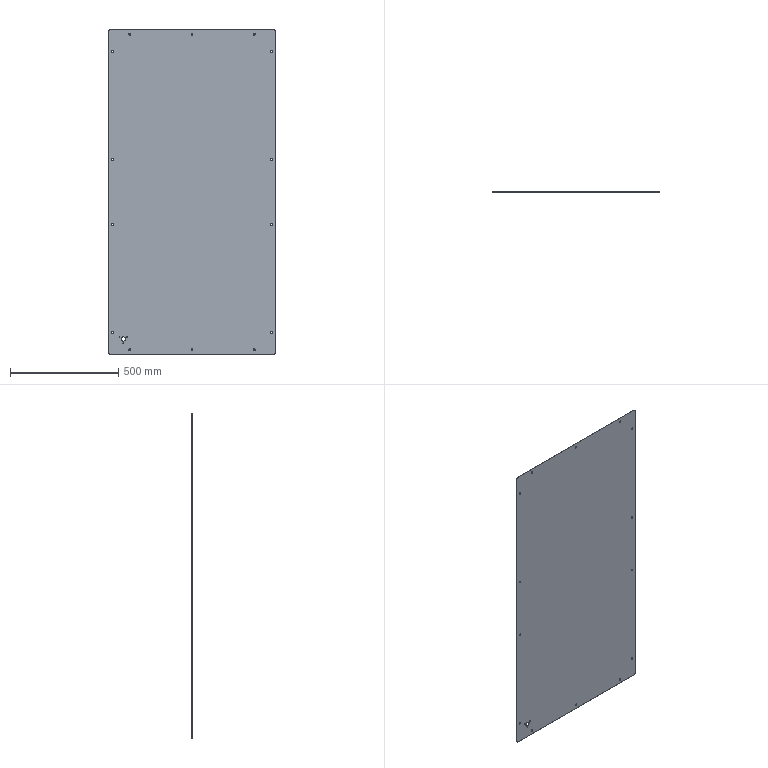Part | STEP file | 09-07 upper cover (Default) | 1 solid | 46 faces | box 775 x 1.5 x 1500 mm | volume 1741776 mm3 | cylinder 40 | plane 6 | commonest cylinder face diameters 9 x28 3.3 x6 20 x6